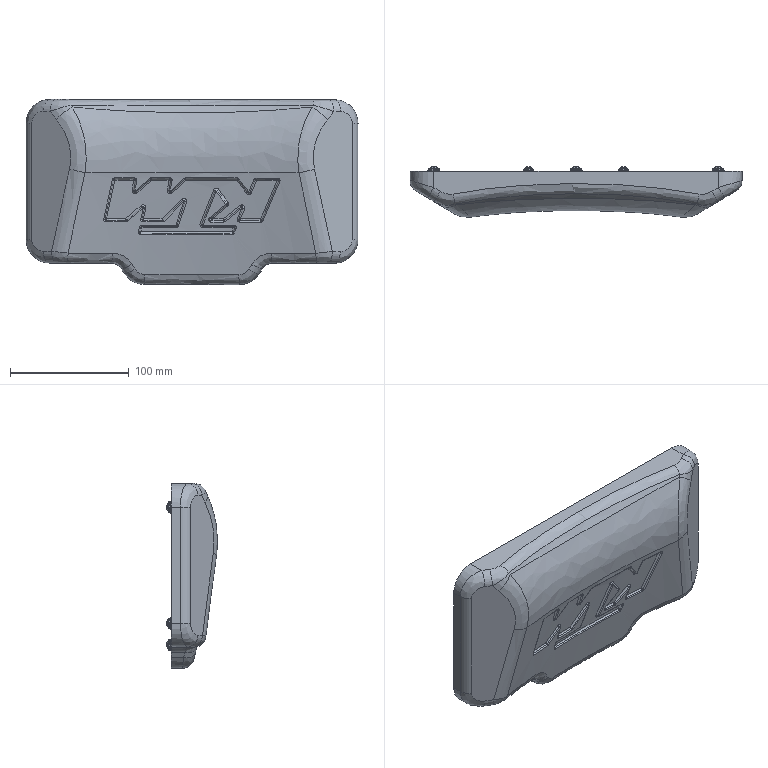Part | SolidWorks | 16 solids | 1552 faces | box 280.077 x 42.75 x 156.126 mm | volume 1225971 mm3 | cylinder 560 | plane 321 | spline 318 | torus 167 | cone 146 | sphere 40 | commonest cylinder face diameters 0.6 x122 4 x112 2 x84 3.4 x42 12 x42 7.4 x28